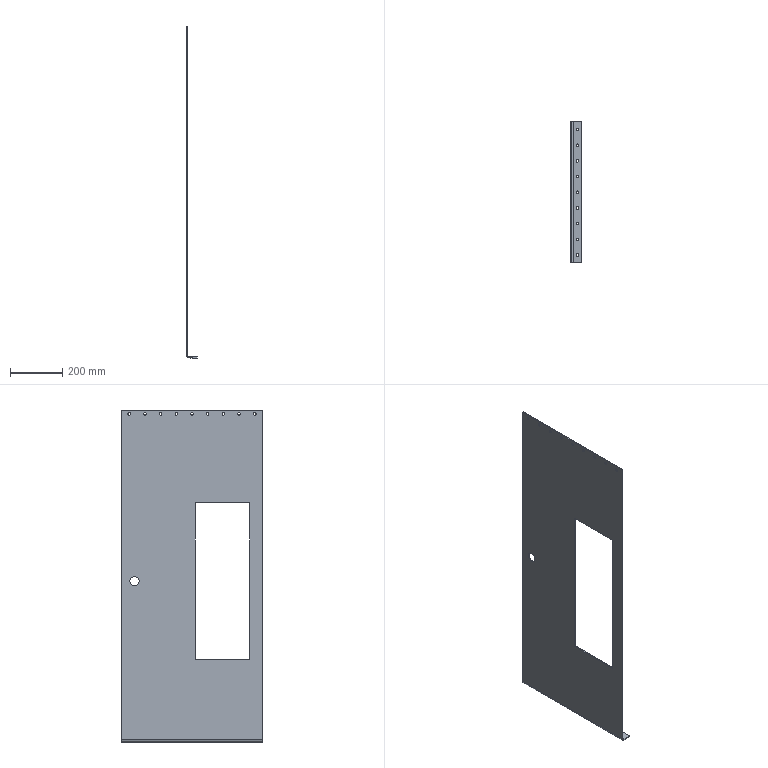Part | SolidWorks | features HoleWzd 2, ICE 2, LPattern 2, Cut 1, EdgeFlange 1, FlatPattern 1, SMBaseFlange 1, SheetMetal 1 | 1 solid | 56 faces | box 40 x 540 x 1270 mm | volume 2305767 mm3 | cylinder 40 | plane 16 | commonest cylinder face diameters 10 x37 35 x2 18 x1